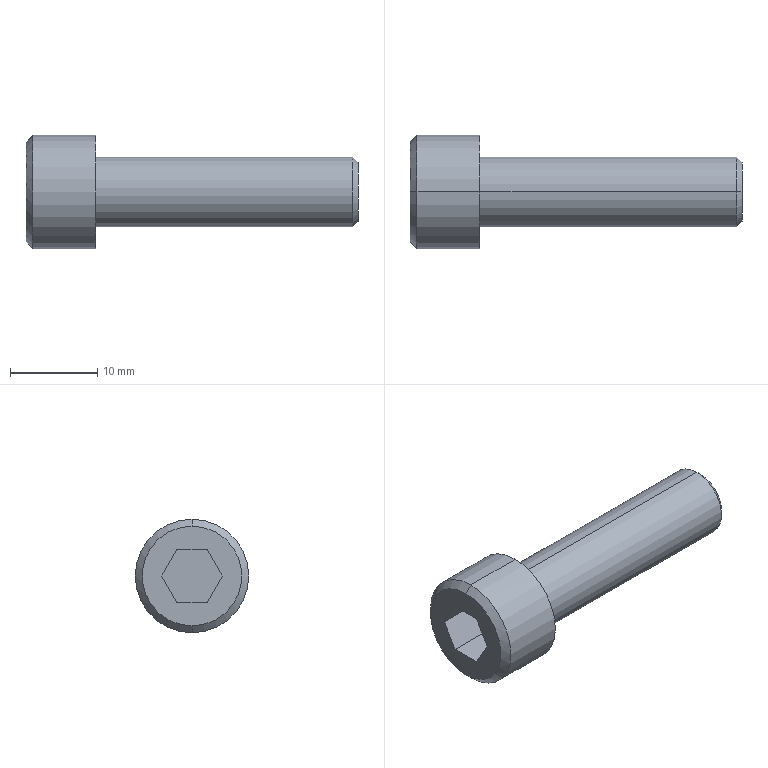Part | Creo | 1 solid | 18 faces | box 38 x 13 x 13 mm | volume 2403 mm3 | plane 10 | cylinder 4 | cone 4 | commonest cylinder face diameters 8 x2 13 x2
STEP:
#1=CARTESIAN_POINT('',(-316.002,-250.,-27.));
#2=VERTEX_POINT('',#1);
#3=CARTESIAN_POINT('',(-316.002,-250.,-40.));
#4=VERTEX_POINT('',#3);
#5=CARTESIAN_POINT('',(-316.002,-250.,-33.5));
#6=DIRECTION('',(1.,0.,0.));
#7=DIRECTION('',(0.,0.,1.));
#8=AXIS2_PLACEMENT_3D('',#5,#6,#7);
#9=CIRCLE('',#8,6.5);
#10=EDGE_CURVE('',#2,#4,#9,.T.);
#11=ORIENTED_EDGE('',*,*,#10,.F.);
#12=CARTESIAN_POINT('',(-316.002,-250.,-33.5));
#13=DIRECTION('',(1.,0.,0.));
#14=DIRECTION('',(0.,0.,-1.));
#15=AXIS2_PLACEMENT_3D('',#12,#13,#14);
#16=CIRCLE('',#15,6.5);
#17=EDGE_CURVE('',#4,#2,#16,.T.);
#18=ORIENTED_EDGE('',*,*,#17,.F.);
#19=EDGE_LOOP('',(#11,#18));
#20=FACE_OUTER_BOUND('',#19,.F.);
#21=CARTESIAN_POINT('',(-316.002,-250.,-37.5));
#22=VERTEX_POINT('',#21);
#23=CARTESIAN_POINT('',(-316.002,-250.,-29.5));
#24=VERTEX_POINT('',#23);
#25=CARTESIAN_POINT('',(-316.002,-250.,-33.5));
#26=DIRECTION('',(-1.,0.,0.));
#27=DIRECTION('',(0.,0.,-1.));
#28=AXIS2_PLACEMENT_3D('',#25,#26,#27);
#29=CIRCLE('',#28,4.);
#30=EDGE_CURVE('',#22,#24,#29,.T.);
#31=ORIENTED_EDGE('',*,*,#30,.F.);
#32=CARTESIAN_POINT('',(-316.002,-250.,-33.5));
#33=DIRECTION('',(-1.,0.,0.));
#34=DIRECTION('',(0.,0.,1.));
#35=AXIS2_PLACEMENT_3D('',#32,#33,#34);
#36=CIRCLE('',#35,4.);
#37=EDGE_CURVE('',#24,#22,#36,.T.);
#38=ORIENTED_EDGE('',*,*,#37,.F.);
#39=EDGE_LOOP('',(#31,#38));
#40=FACE_BOUND('',#39,.F.);
#41=CARTESIAN_POINT('',(-316.002,-250.,-33.5));
#42=DIRECTION('',(1.,0.,0.));
#43=DIRECTION('',(0.,0.,-1.));
#44=AXIS2_PLACEMENT_3D('',#41,#42,#43);
#45=PLANE('',#44);
#46=ADVANCED_FACE('',(#20,#40),#45,.T.);
#47=CARTESIAN_POINT('',(-286.602,-250.,-29.5));
#48=VERTEX_POINT('',#47);
#49=CARTESIAN_POINT('',(-286.602,-250.,-37.5));
#50=VERTEX_POINT('',#49);
#51=CARTESIAN_POINT('',(-286.602,-250.,-33.5));
#52=DIRECTION('',(1.,0.,0.));
#53=DIRECTION('',(0.,0.,1.));
#54=AXIS2_PLACEMENT_3D('',#51,#52,#53);
#55=CIRCLE('',#54,4.);
#56=EDGE_CURVE('',#48,#50,#55,.T.);
#57=ORIENTED_EDGE('',*,*,#56,.T.);
#58=CARTESIAN_POINT('',(-316.002,-250.,-37.5));
#59=DIRECTION('',(1.,0.,0.));
#60=VECTOR('',#59,29.4);
#61=LINE('',#58,#60);
#62=EDGE_CURVE('',#22,#50,#61,.T.);
#63=ORIENTED_EDGE('',*,*,#62,.F.);
#64=ORIENTED_EDGE('',*,*,#30,.T.);
#65=CARTESIAN_POINT('',(-316.002,-250.,-29.5));
#66=DIRECTION('',(1.,0.,0.));
#67=VECTOR('',#66,29.4);
#68=LINE('',#65,#67);
#69=EDGE_CURVE('',#24,#48,#68,.T.);
#70=ORIENTED_EDGE('',*,*,#69,.T.);
#71=EDGE_LOOP('',(#57,#63,#64,#70));
#72=FACE_OUTER_BOUND('',#71,.F.);
#73=CARTESIAN_POINT('',(-320.002,-250.,-33.5));
#74=DIRECTION('',(1.,0.,0.));
#75=DIRECTION('',(0.,0.,-1.));
#76=AXIS2_PLACEMENT_3D('',#73,#74,#75);
#77=CYLINDRICAL_SURFACE('',#76,4.);
#78=ADVANCED_FACE('',(#72),#77,.T.);
#79=CARTESIAN_POINT('',(-286.002,-250.,-30.1));
#80=VERTEX_POINT('',#79);
#81=CARTESIAN_POINT('',(-286.002,-250.,-36.9));
#82=VERTEX_POINT('',#81);
#83=CARTESIAN_POINT('',(-286.002,-250.,-33.5));
#84=DIRECTION('',(1.,0.,0.));
#85=DIRECTION('',(0.,0.,1.));
#86=AXIS2_PLACEMENT_3D('',#83,#84,#85);
#87=CIRCLE('',#86,3.4);
#88=EDGE_CURVE('',#80,#82,#87,.T.);
#89=ORIENTED_EDGE('',*,*,#88,.T.);
#90=CARTESIAN_POINT('',(-286.002,-250.,-36.9));
#91=DIRECTION('',(-0.7071,0.,-0.7071));
#92=VECTOR('',#91,0.8485);
#93=LINE('',#90,#92);
#94=EDGE_CURVE('',#82,#50,#93,.T.);
#95=ORIENTED_EDGE('',*,*,#94,.T.);
#96=ORIENTED_EDGE('',*,*,#56,.F.);
#97=CARTESIAN_POINT('',(-286.002,-250.,-30.1));
#98=DIRECTION('',(-0.7071,0.,0.7071));
#99=VECTOR('',#98,0.8485);
#100=LINE('',#97,#99);
#101=EDGE_CURVE('',#80,#48,#100,.T.);
#102=ORIENTED_EDGE('',*,*,#101,.F.);
#103=EDGE_LOOP('',(#89,#95,#96,#102));
#104=FACE_OUTER_BOUND('',#103,.F.);
#105=CARTESIAN_POINT('',(-286.302,-250.,-33.5));
#106=DIRECTION('',(-1.,0.,0.));
#107=DIRECTION('',(0.,0.,1.));
#108=AXIS2_PLACEMENT_3D('',#105,#106,#107);
#109=CONICAL_SURFACE('',#108,3.7,45.);
#110=ADVANCED_FACE('',(#104),#109,.T.);
#111=CARTESIAN_POINT('',(-286.002,-250.,-33.5));
#112=DIRECTION('',(1.,0.,0.));
#113=DIRECTION('',(0.,0.,-1.));
#114=AXIS2_PLACEMENT_3D('',#111,#112,#113);
#115=CIRCLE('',#114,3.4);
#116=EDGE_CURVE('',#82,#80,#115,.T.);
#117=ORIENTED_EDGE('',*,*,#116,.F.);
#118=ORIENTED_EDGE('',*,*,#88,.F.);
#119=EDGE_LOOP('',(#117,#118));
#120=FACE_OUTER_BOUND('',#119,.F.);
#121=CARTESIAN_POINT('',(-286.002,-250.,-33.5));
#122=DIRECTION('',(1.,0.,0.));
#123=DIRECTION('',(0.,0.,-1.));
#124=AXIS2_PLACEMENT_3D('',#121,#122,#123);
#125=PLANE('',#124);
#126=ADVANCED_FACE('',(#120),#125,.T.);
#127=ORIENTED_EDGE('',*,*,#116,.T.);
#128=ORIENTED_EDGE('',*,*,#101,.T.);
#129=CARTESIAN_POINT('',(-286.602,-250.,-33.5));
#130=DIRECTION('',(1.,0.,0.));
#131=DIRECTION('',(0.,0.,-1.));
#132=AXIS2_PLACEMENT_3D('',#129,#130,#131);
#133=CIRCLE('',#132,4.);
#134=EDGE_CURVE('',#50,#48,#133,.T.);
#135=ORIENTED_EDGE('',*,*,#134,.F.);
#136=ORIENTED_EDGE('',*,*,#94,.F.);
#137=EDGE_LOOP('',(#127,#128,#135,#136));
#138=FACE_OUTER_BOUND('',#137,.F.);
#139=CARTESIAN_POINT('',(-286.302,-250.,-33.5));
#140=DIRECTION('',(-1.,0.,0.));
#141=DIRECTION('',(0.,0.,1.));
#142=AXIS2_PLACEMENT_3D('',#139,#140,#141);
#143=CONICAL_SURFACE('',#142,3.7,45.);
#144=ADVANCED_FACE('',(#138),#143,.T.);
#145=ORIENTED_EDGE('',*,*,#134,.T.);
#146=ORIENTED_EDGE('',*,*,#69,.F.);
#147=ORIENTED_EDGE('',*,*,#37,.T.);
#148=ORIENTED_EDGE('',*,*,#62,.T.);
#149=EDGE_LOOP('',(#145,#146,#147,#148));
#150=FACE_OUTER_BOUND('',#149,.F.);
#151=CARTESIAN_POINT('',(-320.002,-250.,-33.5));
#152=DIRECTION('',(1.,0.,0.));
#153=DIRECTION('',(0.,0.,-1.));
#154=AXIS2_PLACEMENT_3D('',#151,#152,#153);
#155=CYLINDRICAL_SURFACE('',#154,4.);
#156=ADVANCED_FACE('',(#150),#155,.T.);
#157=CARTESIAN_POINT('',(-323.202,-250.,-40.));
#158=VERTEX_POINT('',#157);
#159=CARTESIAN_POINT('',(-323.202,-250.,-27.));
#160=VERTEX_POINT('',#159);
#161=CARTESIAN_POINT('',(-323.202,-250.,-33.5));
#162=DIRECTION('',(-1.,0.,0.));
#163=DIRECTION('',(0.,0.,-1.));
#164=AXIS2_PLACEMENT_3D('',#161,#162,#163);
#165=CIRCLE('',#164,6.5);
#166=EDGE_CURVE('',#158,#160,#165,.T.);
#167=ORIENTED_EDGE('',*,*,#166,.T.);
#168=CARTESIAN_POINT('',(-323.202,-250.,-27.));
#169=DIRECTION('',(1.,0.,0.));
#170=VECTOR('',#169,7.2);
#171=LINE('',#168,#170);
#172=EDGE_CURVE('',#160,#2,#171,.T.);
#173=ORIENTED_EDGE('',*,*,#172,.T.);
#174=ORIENTED_EDGE('',*,*,#10,.T.);
#175=CARTESIAN_POINT('',(-323.202,-250.,-40.));
#176=DIRECTION('',(1.,0.,0.));
#177=VECTOR('',#176,7.2);
#178=LINE('',#175,#177);
#179=EDGE_CURVE('',#158,#4,#178,.T.);
#180=ORIENTED_EDGE('',*,*,#179,.F.);
#181=EDGE_LOOP('',(#167,#173,#174,#180));
#182=FACE_OUTER_BOUND('',#181,.F.);
#183=CARTESIAN_POINT('',(-325.002,-250.,-33.5));
#184=DIRECTION('',(1.,0.,0.));
#185=DIRECTION('',(0.,0.,-1.));
#186=AXIS2_PLACEMENT_3D('',#183,#184,#185);
#187=CYLINDRICAL_SURFACE('',#186,6.5);
#188=ADVANCED_FACE('',(#182),#187,.T.);
#189=CARTESIAN_POINT('',(-324.002,-250.,-39.2));
#190=VERTEX_POINT('',#189);
#191=CARTESIAN_POINT('',(-324.002,-250.,-27.8));
#192=VERTEX_POINT('',#191);
#193=CARTESIAN_POINT('',(-324.002,-250.,-33.5));
#194=DIRECTION('',(-1.,0.,0.));
#195=DIRECTION('',(0.,0.,-1.));
#196=AXIS2_PLACEMENT_3D('',#193,#194,#195);
#197=CIRCLE('',#196,5.7);
#198=EDGE_CURVE('',#190,#192,#197,.T.);
#199=ORIENTED_EDGE('',*,*,#198,.T.);
#200=CARTESIAN_POINT('',(-324.002,-250.,-27.8));
#201=DIRECTION('',(0.7071,0.,0.7071));
#202=VECTOR('',#201,1.131);
#203=LINE('',#200,#202);
#204=EDGE_CURVE('',#192,#160,#203,.T.);
#205=ORIENTED_EDGE('',*,*,#204,.T.);
#206=ORIENTED_EDGE('',*,*,#166,.F.);
#207=CARTESIAN_POINT('',(-324.002,-250.,-39.2));
#208=DIRECTION('',(0.7071,0.,-0.7071));
#209=VECTOR('',#208,1.131);
#210=LINE('',#207,#209);
#211=EDGE_CURVE('',#190,#158,#210,.T.);
#212=ORIENTED_EDGE('',*,*,#211,.F.);
#213=EDGE_LOOP('',(#199,#205,#206,#212));
#214=FACE_OUTER_BOUND('',#213,.F.);
#215=CARTESIAN_POINT('',(-323.602,-250.,-33.5));
#216=DIRECTION('',(1.,0.,0.));
#217=DIRECTION('',(0.,0.,-1.));
#218=AXIS2_PLACEMENT_3D('',#215,#216,#217);
#219=CONICAL_SURFACE('',#218,6.1,45.);
#220=ADVANCED_FACE('',(#214),#219,.T.);
#221=ORIENTED_EDGE('',*,*,#198,.F.);
#222=CARTESIAN_POINT('',(-324.002,-250.,-33.5));
#223=DIRECTION('',(-1.,0.,0.));
#224=DIRECTION('',(0.,0.,1.));
#225=AXIS2_PLACEMENT_3D('',#222,#223,#224);
#226=CIRCLE('',#225,5.7);
#227=EDGE_CURVE('',#192,#190,#226,.T.);
#228=ORIENTED_EDGE('',*,*,#227,.F.);
#229=EDGE_LOOP('',(#221,#228));
#230=FACE_OUTER_BOUND('',#229,.F.);
#231=CARTESIAN_POINT('',(-324.002,-251.732,-30.5));
#232=VERTEX_POINT('',#231);
#233=CARTESIAN_POINT('',(-324.002,-253.464,-33.5));
#234=VERTEX_POINT('',#233);
#235=CARTESIAN_POINT('',(-324.002,-251.732,-30.5));
#236=DIRECTION('',(0.,-0.5,-0.866));
#237=VECTOR('',#236,3.464);
#238=LINE('',#235,#237);
#239=EDGE_CURVE('',#232,#234,#238,.T.);
#240=ORIENTED_EDGE('',*,*,#239,.F.);
#241=CARTESIAN_POINT('',(-324.002,-248.268,-30.5));
#242=VERTEX_POINT('',#241);
#243=CARTESIAN_POINT('',(-324.002,-248.268,-30.5));
#244=DIRECTION('',(0.,-1.,0.));
#245=VECTOR('',#244,3.464);
#246=LINE('',#243,#245);
#247=EDGE_CURVE('',#242,#232,#246,.T.);
#248=ORIENTED_EDGE('',*,*,#247,.F.);
#249=CARTESIAN_POINT('',(-324.002,-246.536,-33.5));
#250=VERTEX_POINT('',#249);
#251=CARTESIAN_POINT('',(-324.002,-246.536,-33.5));
#252=DIRECTION('',(0.,-0.5,0.866));
#253=VECTOR('',#252,3.464);
#254=LINE('',#251,#253);
#255=EDGE_CURVE('',#250,#242,#254,.T.);
#256=ORIENTED_EDGE('',*,*,#255,.F.);
#257=CARTESIAN_POINT('',(-324.002,-248.268,-36.5));
#258=VERTEX_POINT('',#257);
#259=CARTESIAN_POINT('',(-324.002,-248.268,-36.5));
#260=DIRECTION('',(0.,0.5,0.866));
#261=VECTOR('',#260,3.464);
#262=LINE('',#259,#261);
#263=EDGE_CURVE('',#258,#250,#262,.T.);
#264=ORIENTED_EDGE('',*,*,#263,.F.);
#265=CARTESIAN_POINT('',(-324.002,-251.732,-36.5));
#266=VERTEX_POINT('',#265);
#267=CARTESIAN_POINT('',(-324.002,-251.732,-36.5));
#268=DIRECTION('',(0.,1.,0.));
#269=VECTOR('',#268,3.464);
#270=LINE('',#267,#269);
#271=EDGE_CURVE('',#266,#258,#270,.T.);
#272=ORIENTED_EDGE('',*,*,#271,.F.);
#273=CARTESIAN_POINT('',(-324.002,-253.464,-33.5));
#274=DIRECTION('',(0.,0.5,-0.866));
#275=VECTOR('',#274,3.464);
#276=LINE('',#273,#275);
#277=EDGE_CURVE('',#234,#266,#276,.T.);
#278=ORIENTED_EDGE('',*,*,#277,.F.);
#279=EDGE_LOOP('',(#240,#248,#256,#264,#272,#278));
#280=FACE_BOUND('',#279,.F.);
#281=CARTESIAN_POINT('',(-324.002,-250.,-33.5));
#282=DIRECTION('',(1.,0.,0.));
#283=DIRECTION('',(0.,0.,-1.));
#284=AXIS2_PLACEMENT_3D('',#281,#282,#283);
#285=PLANE('',#284);
#286=ADVANCED_FACE('',(#230,#280),#285,.F.);
#287=ORIENTED_EDGE('',*,*,#227,.T.);
#288=ORIENTED_EDGE('',*,*,#211,.T.);
#289=CARTESIAN_POINT('',(-323.202,-250.,-33.5));
#290=DIRECTION('',(-1.,0.,0.));
#291=DIRECTION('',(0.,0.,1.));
#292=AXIS2_PLACEMENT_3D('',#289,#290,#291);
#293=CIRCLE('',#292,6.5);
#294=EDGE_CURVE('',#160,#158,#293,.T.);
#295=ORIENTED_EDGE('',*,*,#294,.F.);
#296=ORIENTED_EDGE('',*,*,#204,.F.);
#297=EDGE_LOOP('',(#287,#288,#295,#296));
#298=FACE_OUTER_BOUND('',#297,.F.);
#299=CARTESIAN_POINT('',(-323.602,-250.,-33.5));
#300=DIRECTION('',(1.,0.,0.));
#301=DIRECTION('',(0.,0.,-1.));
#302=AXIS2_PLACEMENT_3D('',#299,#300,#301);
#303=CONICAL_SURFACE('',#302,6.1,45.);
#304=ADVANCED_FACE('',(#298),#303,.T.);
#305=ORIENTED_EDGE('',*,*,#294,.T.);
#306=ORIENTED_EDGE('',*,*,#179,.T.);
#307=ORIENTED_EDGE('',*,*,#17,.T.);
#308=ORIENTED_EDGE('',*,*,#172,.F.);
#309=EDGE_LOOP('',(#305,#306,#307,#308));
#310=FACE_OUTER_BOUND('',#309,.F.);
#311=CARTESIAN_POINT('',(-325.002,-250.,-33.5));
#312=DIRECTION('',(1.,0.,0.));
#313=DIRECTION('',(0.,0.,-1.));
#314=AXIS2_PLACEMENT_3D('',#311,#312,#313);
#315=CYLINDRICAL_SURFACE('',#314,6.5);
#316=ADVANCED_FACE('',(#310),#315,.T.);
#317=ORIENTED_EDGE('',*,*,#239,.T.);
#318=CARTESIAN_POINT('',(-319.202,-253.464,-33.5));
#319=VERTEX_POINT('',#318);
#320=CARTESIAN_POINT('',(-324.002,-253.464,-33.5));
#321=DIRECTION('',(1.,0.,0.));
#322=VECTOR('',#321,4.8);
#323=LINE('',#320,#322);
#324=EDGE_CURVE('',#234,#319,#323,.T.);
#325=ORIENTED_EDGE('',*,*,#324,.T.);
#326=CARTESIAN_POINT('',(-319.202,-251.732,-30.5));
#327=VERTEX_POINT('',#326);
#328=CARTESIAN_POINT('',(-319.202,-253.464,-33.5));
#329=DIRECTION('',(0.,0.5,0.866));
#330=VECTOR('',#329,3.464);
#331=LINE('',#328,#330);
#332=EDGE_CURVE('',#319,#327,#331,.T.);
#333=ORIENTED_EDGE('',*,*,#332,.T.);
#334=CARTESIAN_POINT('',(-324.002,-251.732,-30.5));
#335=DIRECTION('',(1.,0.,0.));
#336=VECTOR('',#335,4.8);
#337=LINE('',#334,#336);
#338=EDGE_CURVE('',#232,#327,#337,.T.);
#339=ORIENTED_EDGE('',*,*,#338,.F.);
#340=EDGE_LOOP('',(#317,#325,#333,#339));
#341=FACE_OUTER_BOUND('',#340,.F.);
#342=CARTESIAN_POINT('',(-319.202,-253.464,-33.5));
#343=DIRECTION('',(0.,-0.866,0.5));
#344=DIRECTION('',(0.,-0.5,-0.866));
#345=AXIS2_PLACEMENT_3D('',#342,#343,#344);
#346=PLANE('',#345);
#347=ADVANCED_FACE('',(#341),#346,.F.);
#348=ORIENTED_EDGE('',*,*,#277,.T.);
#349=CARTESIAN_POINT('',(-319.202,-251.732,-36.5));
#350=VERTEX_POINT('',#349);
#351=CARTESIAN_POINT('',(-324.002,-251.732,-36.5));
#352=DIRECTION('',(1.,0.,0.));
#353=VECTOR('',#352,4.8);
#354=LINE('',#351,#353);
#355=EDGE_CURVE('',#266,#350,#354,.T.);
#356=ORIENTED_EDGE('',*,*,#355,.T.);
#357=CARTESIAN_POINT('',(-319.202,-251.732,-36.5));
#358=DIRECTION('',(0.,-0.5,0.866));
#359=VECTOR('',#358,3.464);
#360=LINE('',#357,#359);
#361=EDGE_CURVE('',#350,#319,#360,.T.);
#362=ORIENTED_EDGE('',*,*,#361,.T.);
#363=ORIENTED_EDGE('',*,*,#324,.F.);
#364=EDGE_LOOP('',(#348,#356,#362,#363));
#365=FACE_OUTER_BOUND('',#364,.F.);
#366=CARTESIAN_POINT('',(-319.202,-251.732,-36.5));
#367=DIRECTION('',(0.,-0.866,-0.5));
#368=DIRECTION('',(0.,0.5,-0.866));
#369=AXIS2_PLACEMENT_3D('',#366,#367,#368);
#370=PLANE('',#369);
#371=ADVANCED_FACE('',(#365),#370,.F.);
#372=ORIENTED_EDGE('',*,*,#271,.T.);
#373=CARTESIAN_POINT('',(-319.202,-248.268,-36.5));
#374=VERTEX_POINT('',#373);
#375=CARTESIAN_POINT('',(-324.002,-248.268,-36.5));
#376=DIRECTION('',(1.,0.,0.));
#377=VECTOR('',#376,4.8);
#378=LINE('',#375,#377);
#379=EDGE_CURVE('',#258,#374,#378,.T.);
#380=ORIENTED_EDGE('',*,*,#379,.T.);
#381=CARTESIAN_POINT('',(-319.202,-251.732,-36.5));
#382=DIRECTION('',(0.,1.,0.));
#383=VECTOR('',#382,3.464);
#384=LINE('',#381,#383);
#385=EDGE_CURVE('',#350,#374,#384,.T.);
#386=ORIENTED_EDGE('',*,*,#385,.F.);
#387=ORIENTED_EDGE('',*,*,#355,.F.);
#388=EDGE_LOOP('',(#372,#380,#386,#387));
#389=FACE_OUTER_BOUND('',#388,.F.);
#390=CARTESIAN_POINT('',(-319.202,-248.268,-36.5));
#391=DIRECTION('',(0.,0.,-1.));
#392=DIRECTION('',(-1.,0.,0.));
#393=AXIS2_PLACEMENT_3D('',#390,#391,#392);
#394=PLANE('',#393);
#395=ADVANCED_FACE('',(#389),#394,.F.);
#396=ORIENTED_EDGE('',*,*,#263,.T.);
#397=CARTESIAN_POINT('',(-319.202,-246.536,-33.5));
#398=VERTEX_POINT('',#397);
#399=CARTESIAN_POINT('',(-324.002,-246.536,-33.5));
#400=DIRECTION('',(1.,0.,0.));
#401=VECTOR('',#400,4.8);
#402=LINE('',#399,#401);
#403=EDGE_CURVE('',#250,#398,#402,.T.);
#404=ORIENTED_EDGE('',*,*,#403,.T.);
#405=CARTESIAN_POINT('',(-319.202,-246.536,-33.5));
#406=DIRECTION('',(0.,-0.5,-0.866));
#407=VECTOR('',#406,3.464);
#408=LINE('',#405,#407);
#409=EDGE_CURVE('',#398,#374,#408,.T.);
#410=ORIENTED_EDGE('',*,*,#409,.T.);
#411=ORIENTED_EDGE('',*,*,#379,.F.);
#412=EDGE_LOOP('',(#396,#404,#410,#411));
#413=FACE_OUTER_BOUND('',#412,.F.);
#414=CARTESIAN_POINT('',(-319.202,-246.536,-33.5));
#415=DIRECTION('',(0.,0.866,-0.5));
#416=DIRECTION('',(0.,0.5,0.866));
#417=AXIS2_PLACEMENT_3D('',#414,#415,#416);
#418=PLANE('',#417);
#419=ADVANCED_FACE('',(#413),#418,.F.);
#420=ORIENTED_EDGE('',*,*,#255,.T.);
#421=CARTESIAN_POINT('',(-319.202,-248.268,-30.5));
#422=VERTEX_POINT('',#421);
#423=CARTESIAN_POINT('',(-324.002,-248.268,-30.5));
#424=DIRECTION('',(1.,0.,0.));
#425=VECTOR('',#424,4.8);
#426=LINE('',#423,#425);
#427=EDGE_CURVE('',#242,#422,#426,.T.);
#428=ORIENTED_EDGE('',*,*,#427,.T.);
#429=CARTESIAN_POINT('',(-319.202,-248.268,-30.5));
#430=DIRECTION('',(0.,0.5,-0.866));
#431=VECTOR('',#430,3.464);
#432=LINE('',#429,#431);
#433=EDGE_CURVE('',#422,#398,#432,.T.);
#434=ORIENTED_EDGE('',*,*,#433,.T.);
#435=ORIENTED_EDGE('',*,*,#403,.F.);
#436=EDGE_LOOP('',(#420,#428,#434,#435));
#437=FACE_OUTER_BOUND('',#436,.F.);
#438=CARTESIAN_POINT('',(-319.202,-248.268,-30.5));
#439=DIRECTION('',(0.,0.866,0.5));
#440=DIRECTION('',(0.,-0.5,0.866));
#441=AXIS2_PLACEMENT_3D('',#438,#439,#440);
#442=PLANE('',#441);
#443=ADVANCED_FACE('',(#437),#442,.F.);
#444=ORIENTED_EDGE('',*,*,#247,.T.);
#445=ORIENTED_EDGE('',*,*,#338,.T.);
#446=CARTESIAN_POINT('',(-319.202,-248.268,-30.5));
#447=DIRECTION('',(0.,-1.,0.));
#448=VECTOR('',#447,3.464);
#449=LINE('',#446,#448);
#450=EDGE_CURVE('',#422,#327,#449,.T.);
#451=ORIENTED_EDGE('',*,*,#450,.F.);
#452=ORIENTED_EDGE('',*,*,#427,.F.);
#453=EDGE_LOOP('',(#444,#445,#451,#452));
#454=FACE_OUTER_BOUND('',#453,.F.);
#455=CARTESIAN_POINT('',(-319.202,-251.732,-30.5));
#456=DIRECTION('',(0.,0.,1.));
#457=DIRECTION('',(1.,0.,0.));
#458=AXIS2_PLACEMENT_3D('',#455,#456,#457);
#459=PLANE('',#458);
#460=ADVANCED_FACE('',(#454),#459,.F.);
#461=ORIENTED_EDGE('',*,*,#361,.F.);
#462=ORIENTED_EDGE('',*,*,#385,.T.);
#463=ORIENTED_EDGE('',*,*,#409,.F.);
#464=ORIENTED_EDGE('',*,*,#433,.F.);
#465=ORIENTED_EDGE('',*,*,#450,.T.);
#466=ORIENTED_EDGE('',*,*,#332,.F.);
#467=EDGE_LOOP('',(#461,#462,#463,#464,#465,#466));
#468=FACE_OUTER_BOUND('',#467,.F.);
#469=CARTESIAN_POINT('',(-319.202,-250.,-39.5));
#470=DIRECTION('',(1.,0.,0.));
#471=DIRECTION('',(0.,0.,-1.));
#472=AXIS2_PLACEMENT_3D('',#469,#470,#471);
#473=PLANE('',#472);
#474=ADVANCED_FACE('',(#468),#473,.F.);
#475=CLOSED_SHELL('',(#46,#78,#110,#126,#144,#156,#188,#220,#286,#304,#316,#347,#371,#395,#419,#443,#460,#474));
#476=MANIFOLD_SOLID_BREP('',#475);
#477=(LENGTH_UNIT()NAMED_UNIT(*)SI_UNIT(.MILLI.,.METRE.));
#478=UNCERTAINTY_MEASURE_WITH_UNIT(LENGTH_MEASURE(0.004222),#477,'','');
#479=(NAMED_UNIT(*)PLANE_ANGLE_UNIT()SI_UNIT($,.RADIAN.));
#480=PLANE_ANGLE_MEASURE_WITH_UNIT(PLANE_ANGLE_MEASURE(0.01745),#479);
#481=(CONVERSION_BASED_UNIT('DEGREE',#480)NAMED_UNIT(*)PLANE_ANGLE_UNIT());
#482=(NAMED_UNIT(*)SI_UNIT($,.STERADIAN.)SOLID_ANGLE_UNIT());
#483=(GEOMETRIC_REPRESENTATION_CONTEXT(3)GLOBAL_UNCERTAINTY_ASSIGNED_CONTEXT((#478))GLOBAL_UNIT_ASSIGNED_CONTEXT((#477,#481,#482))REPRESENTATION_CONTEXT('',''));
#484=ADVANCED_BREP_SHAPE_REPRESENTATION('',(#476),#483);